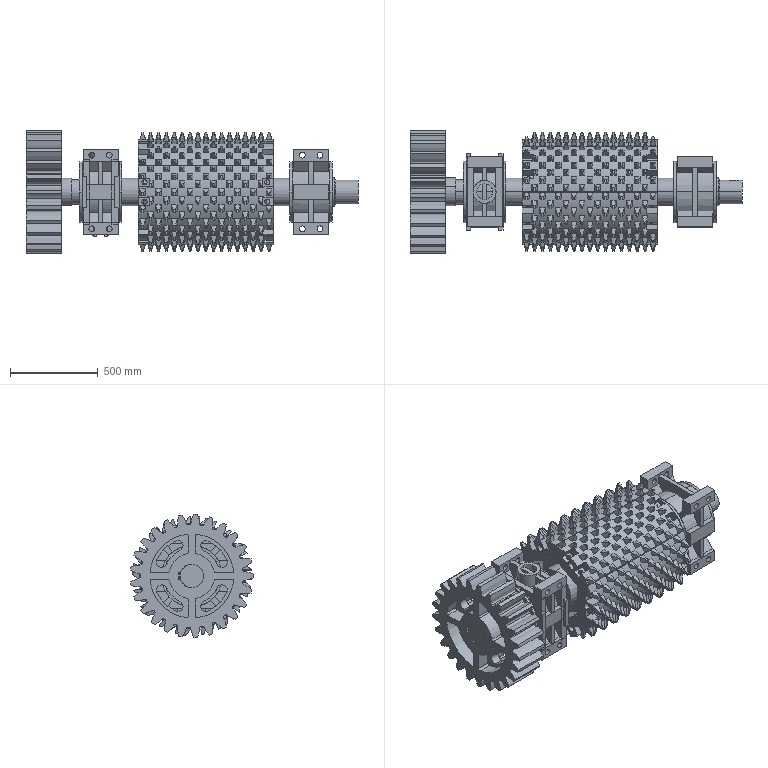Part | NX | features BREP 14, MOVE_FACE 4, DATUM_CSYS 3, SKETCH 3 | 28 solids | 4666 faces | volume 267145378 mm3 | plane 3005 | cylinder 1175 | cone 398 | spline 50 | torus 38 | commonest cylinder face diameters 38 x345 30 x96 20 x88 16 x72 10 x48 18 x48